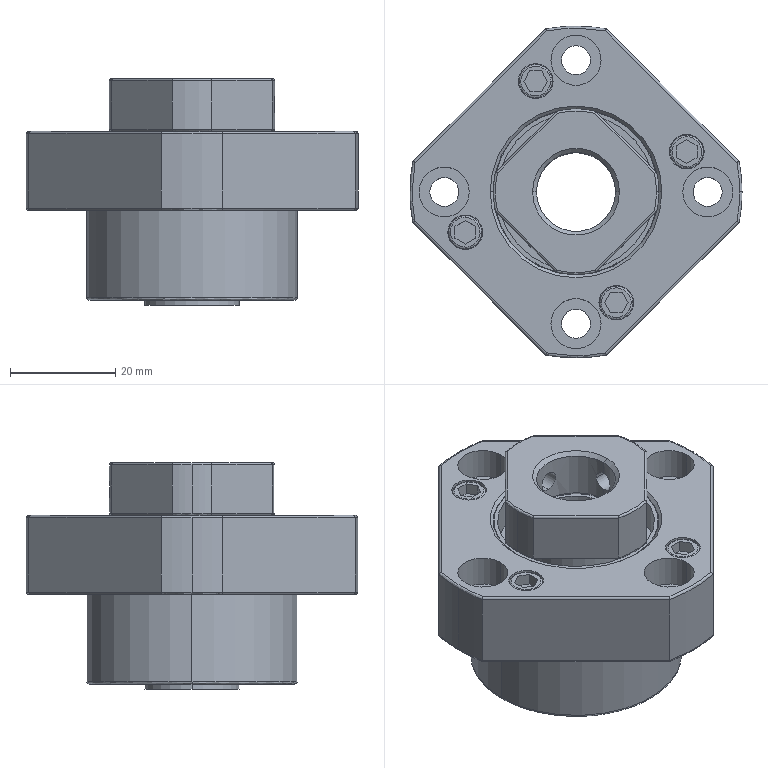Part | STEP file | 001-010-ZS-FK15 | 7 solids | 199 faces | box 63 x 63 x 43 mm | volume 52330 mm3 | cylinder 92 | plane 65 | spline 30 | cone 12 | commonest cylinder face diameters 0.75 x8 0.9 x8 5.5 x8 6.265 x8 6.578 x8 9.5 x8